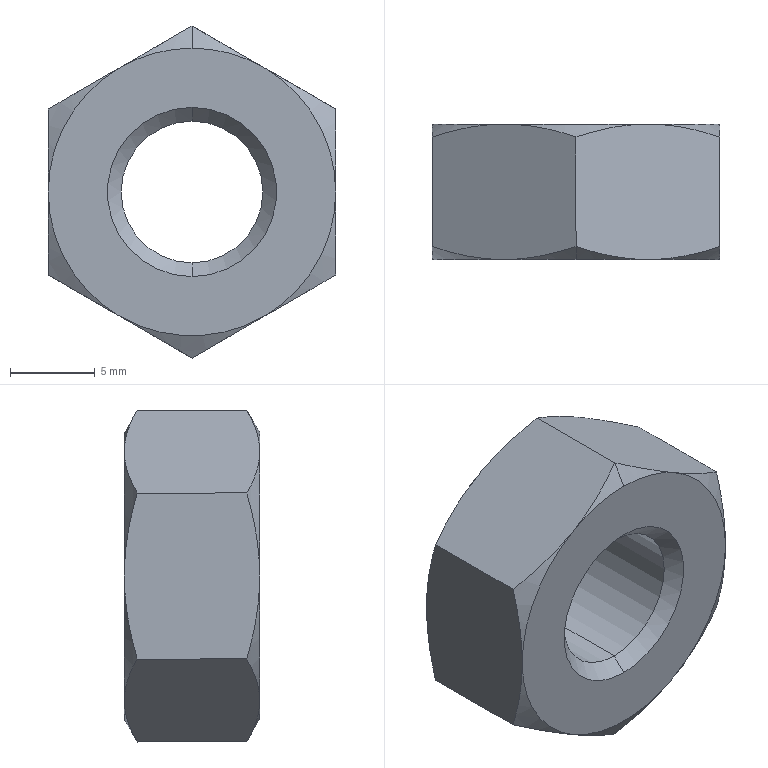Part | SolidWorks | features BaseBody 1 | 1 solid | 27 faces | box 17 x 8 x 19.63 mm | volume 1532 mm3 | cone 17 | plane 8 | cylinder 2 | commonest cylinder face diameters 8.376 x2
STEP:
#1=CARTESIAN_POINT('',(0.,0.812,-4.188));
#2=VERTEX_POINT('',#1);
#3=CARTESIAN_POINT('',(0.,0.812,4.188));
#4=VERTEX_POINT('',#3);
#5=CARTESIAN_POINT('',(0.,0.812,0.));
#6=DIRECTION('',(0.,1.,0.));
#7=DIRECTION('',(0.,0.,1.));
#8=AXIS2_PLACEMENT_3D('',#5,#6,#7);
#9=CIRCLE('',#8,4.188);
#10=EDGE_CURVE('',#2,#4,#9,.T.);
#11=ORIENTED_EDGE('',*,*,#10,.F.);
#12=CARTESIAN_POINT('',(0.,7.188,-4.188));
#13=VERTEX_POINT('',#12);
#14=CARTESIAN_POINT('',(0.,0.,-4.188));
#15=DIRECTION('',(0.,1.,0.));
#16=VECTOR('',#15,1000.);
#17=LINE('',#14,#16);
#18=EDGE_CURVE('',#2,#13,#17,.T.);
#19=ORIENTED_EDGE('',*,*,#18,.T.);
#20=CARTESIAN_POINT('',(0.,7.188,4.188));
#21=VERTEX_POINT('',#20);
#22=CARTESIAN_POINT('',(0.,7.188,0.));
#23=DIRECTION('',(0.,-1.,0.));
#24=DIRECTION('',(0.,0.,1.));
#25=AXIS2_PLACEMENT_3D('',#22,#23,#24);
#26=CIRCLE('',#25,4.188);
#27=EDGE_CURVE('',#21,#13,#26,.T.);
#28=ORIENTED_EDGE('',*,*,#27,.F.);
#29=CARTESIAN_POINT('',(0.,0.,4.188));
#30=DIRECTION('',(0.,1.,0.));
#31=VECTOR('',#30,1000.);
#32=LINE('',#29,#31);
#33=EDGE_CURVE('',#4,#21,#32,.T.);
#34=ORIENTED_EDGE('',*,*,#33,.F.);
#35=EDGE_LOOP('',(#11,#19,#28,#34));
#36=FACE_OUTER_BOUND('',#35,.T.);
#37=CARTESIAN_POINT('',(0.,0.,0.));
#38=DIRECTION('',(0.,1.,0.));
#39=DIRECTION('',(0.,0.,1.));
#40=AXIS2_PLACEMENT_3D('',#37,#38,#39);
#41=CYLINDRICAL_SURFACE('',#40,4.188);
#42=ADVANCED_FACE('',(#36),#41,.F.);
#43=ORIENTED_EDGE('',*,*,#27,.T.);
#44=CARTESIAN_POINT('',(0.,8.,-5.));
#45=VERTEX_POINT('',#44);
#46=CARTESIAN_POINT('',(0.,8.,-5.));
#47=DIRECTION('',(0.,0.7071,-0.7071));
#48=VECTOR('',#47,1000.);
#49=LINE('',#46,#48);
#50=EDGE_CURVE('',#13,#45,#49,.T.);
#51=ORIENTED_EDGE('',*,*,#50,.T.);
#52=CARTESIAN_POINT('',(0.,8.,5.));
#53=VERTEX_POINT('',#52);
#54=CARTESIAN_POINT('',(0.,8.,0.));
#55=DIRECTION('',(0.,-1.,0.));
#56=DIRECTION('',(0.,0.,1.));
#57=AXIS2_PLACEMENT_3D('',#54,#55,#56);
#58=CIRCLE('',#57,5.);
#59=EDGE_CURVE('',#53,#45,#58,.T.);
#60=ORIENTED_EDGE('',*,*,#59,.F.);
#61=CARTESIAN_POINT('',(0.,8.,5.));
#62=DIRECTION('',(0.,0.7071,0.7071));
#63=VECTOR('',#62,1000.);
#64=LINE('',#61,#63);
#65=EDGE_CURVE('',#21,#53,#64,.T.);
#66=ORIENTED_EDGE('',*,*,#65,.F.);
#67=EDGE_LOOP('',(#43,#51,#60,#66));
#68=FACE_OUTER_BOUND('',#67,.T.);
#69=CARTESIAN_POINT('',(0.,8.,0.));
#70=DIRECTION('',(0.,1.,0.));
#71=DIRECTION('',(0.,0.,1.));
#72=AXIS2_PLACEMENT_3D('',#69,#70,#71);
#73=CONICAL_SURFACE('',#72,5.,0.7854);
#74=ADVANCED_FACE('',(#68),#73,.F.);
#75=ORIENTED_EDGE('',*,*,#10,.T.);
#76=CARTESIAN_POINT('',(0.,0.,5.));
#77=VERTEX_POINT('',#76);
#78=CARTESIAN_POINT('',(0.,0.,5.));
#79=DIRECTION('',(0.,-0.7071,0.7071));
#80=VECTOR('',#79,1000.);
#81=LINE('',#78,#80);
#82=EDGE_CURVE('',#4,#77,#81,.T.);
#83=ORIENTED_EDGE('',*,*,#82,.T.);
#84=CARTESIAN_POINT('',(0.,0.,-5.));
#85=VERTEX_POINT('',#84);
#86=CARTESIAN_POINT('',(0.,0.,0.));
#87=DIRECTION('',(0.,1.,0.));
#88=DIRECTION('',(0.,0.,-1.));
#89=AXIS2_PLACEMENT_3D('',#86,#87,#88);
#90=CIRCLE('',#89,5.);
#91=EDGE_CURVE('',#85,#77,#90,.T.);
#92=ORIENTED_EDGE('',*,*,#91,.F.);
#93=CARTESIAN_POINT('',(0.,0.,-5.));
#94=DIRECTION('',(0.,-0.7071,-0.7071));
#95=VECTOR('',#94,1000.);
#96=LINE('',#93,#95);
#97=EDGE_CURVE('',#2,#85,#96,.T.);
#98=ORIENTED_EDGE('',*,*,#97,.F.);
#99=EDGE_LOOP('',(#75,#83,#92,#98));
#100=FACE_OUTER_BOUND('',#99,.T.);
#101=CARTESIAN_POINT('',(0.,0.,0.));
#102=DIRECTION('',(0.,-1.,0.));
#103=DIRECTION('',(0.,0.,-1.));
#104=AXIS2_PLACEMENT_3D('',#101,#102,#103);
#105=CONICAL_SURFACE('',#104,5.,0.7854);
#106=ADVANCED_FACE('',(#100),#105,.F.);
#107=CARTESIAN_POINT('',(-4.25,0.,7.361));
#108=VERTEX_POINT('',#107);
#109=CARTESIAN_POINT('',(0.,0.,8.5));
#110=VERTEX_POINT('',#109);
#111=CARTESIAN_POINT('',(0.,0.,0.));
#112=DIRECTION('',(0.,1.,0.));
#113=DIRECTION('',(0.,0.,1.));
#114=AXIS2_PLACEMENT_3D('',#111,#112,#113);
#115=CIRCLE('',#114,8.5);
#116=EDGE_CURVE('',#108,#110,#115,.T.);
#117=ORIENTED_EDGE('',*,*,#116,.T.);
#118=CARTESIAN_POINT('',(0.000000007,0.7592,9.815));
#119=VERTEX_POINT('',#118);
#120=CARTESIAN_POINT('',(0.,0.7637,9.823));
#121=DIRECTION('',(0.,0.5,0.866));
#122=VECTOR('',#121,1000.);
#123=LINE('',#120,#122);
#124=EDGE_CURVE('',#110,#119,#123,.T.);
#125=ORIENTED_EDGE('',*,*,#124,.T.);
#126=CARTESIAN_POINT('',(0.000000007,0.7592,9.815));
#127=CARTESIAN_POINT('',(-0.6943,0.5278,9.414));
#128=CARTESIAN_POINT('',(-1.394,0.3369,9.01));
#129=CARTESIAN_POINT('',(-2.809,0.07258,8.193));
#130=CARTESIAN_POINT('',(-3.525,0.,7.78));
#131=CARTESIAN_POINT('',(-4.25,0.,7.361));
#132=B_SPLINE_CURVE_WITH_KNOTS('',3,(#126,#127,#128,#129,#130,#131),.UNSPECIFIED.,.F.,.F.,(4,2,4),(0.,0.002483,0.004966),.UNSPECIFIED.);
#133=EDGE_CURVE('',#119,#108,#132,.T.);
#134=ORIENTED_EDGE('',*,*,#133,.T.);
#135=EDGE_LOOP('',(#117,#125,#134));
#136=FACE_OUTER_BOUND('',#135,.T.);
#137=CARTESIAN_POINT('',(0.,0.7637,0.));
#138=DIRECTION('',(0.,1.,0.));
#139=DIRECTION('',(0.,0.,1.));
#140=AXIS2_PLACEMENT_3D('',#137,#138,#139);
#141=CONICAL_SURFACE('',#140,9.823,1.047);
#142=ADVANCED_FACE('',(#136),#141,.T.);
#143=ORIENTED_EDGE('',*,*,#18,.F.);
#144=CARTESIAN_POINT('',(0.,0.812,0.));
#145=DIRECTION('',(0.,1.,0.));
#146=DIRECTION('',(0.,0.,1.));
#147=AXIS2_PLACEMENT_3D('',#144,#145,#146);
#148=CIRCLE('',#147,4.188);
#149=EDGE_CURVE('',#4,#2,#148,.T.);
#150=ORIENTED_EDGE('',*,*,#149,.F.);
#151=ORIENTED_EDGE('',*,*,#33,.T.);
#152=CARTESIAN_POINT('',(0.,7.188,0.));
#153=DIRECTION('',(0.,-1.,0.));
#154=DIRECTION('',(0.,0.,1.));
#155=AXIS2_PLACEMENT_3D('',#152,#153,#154);
#156=CIRCLE('',#155,4.188);
#157=EDGE_CURVE('',#13,#21,#156,.T.);
#158=ORIENTED_EDGE('',*,*,#157,.F.);
#159=EDGE_LOOP('',(#143,#150,#151,#158));
#160=FACE_OUTER_BOUND('',#159,.T.);
#161=CARTESIAN_POINT('',(0.,0.,0.));
#162=DIRECTION('',(0.,1.,0.));
#163=DIRECTION('',(0.,0.,1.));
#164=AXIS2_PLACEMENT_3D('',#161,#162,#163);
#165=CYLINDRICAL_SURFACE('',#164,4.188);
#166=ADVANCED_FACE('',(#160),#165,.F.);
#167=ORIENTED_EDGE('',*,*,#50,.F.);
#168=ORIENTED_EDGE('',*,*,#157,.T.);
#169=ORIENTED_EDGE('',*,*,#65,.T.);
#170=CARTESIAN_POINT('',(0.,8.,0.));
#171=DIRECTION('',(0.,-1.,0.));
#172=DIRECTION('',(0.,0.,1.));
#173=AXIS2_PLACEMENT_3D('',#170,#171,#172);
#174=CIRCLE('',#173,5.);
#175=EDGE_CURVE('',#45,#53,#174,.T.);
#176=ORIENTED_EDGE('',*,*,#175,.F.);
#177=EDGE_LOOP('',(#167,#168,#169,#176));
#178=FACE_OUTER_BOUND('',#177,.T.);
#179=CARTESIAN_POINT('',(0.,8.,0.));
#180=DIRECTION('',(0.,1.,0.));
#181=DIRECTION('',(0.,0.,1.));
#182=AXIS2_PLACEMENT_3D('',#179,#180,#181);
#183=CONICAL_SURFACE('',#182,5.,0.7854);
#184=ADVANCED_FACE('',(#178),#183,.F.);
#185=ORIENTED_EDGE('',*,*,#82,.F.);
#186=ORIENTED_EDGE('',*,*,#149,.T.);
#187=ORIENTED_EDGE('',*,*,#97,.T.);
#188=CARTESIAN_POINT('',(0.,0.,0.));
#189=DIRECTION('',(0.,1.,0.));
#190=DIRECTION('',(0.,0.,-1.));
#191=AXIS2_PLACEMENT_3D('',#188,#189,#190);
#192=CIRCLE('',#191,5.);
#193=EDGE_CURVE('',#77,#85,#192,.T.);
#194=ORIENTED_EDGE('',*,*,#193,.F.);
#195=EDGE_LOOP('',(#185,#186,#187,#194));
#196=FACE_OUTER_BOUND('',#195,.T.);
#197=CARTESIAN_POINT('',(0.,0.,0.));
#198=DIRECTION('',(0.,-1.,0.));
#199=DIRECTION('',(0.,0.,-1.));
#200=AXIS2_PLACEMENT_3D('',#197,#198,#199);
#201=CONICAL_SURFACE('',#200,5.,0.7854);
#202=ADVANCED_FACE('',(#196),#201,.F.);
#203=ORIENTED_EDGE('',*,*,#59,.T.);
#204=ORIENTED_EDGE('',*,*,#175,.T.);
#205=EDGE_LOOP('',(#203,#204));
#206=FACE_BOUND('',#205,.T.);
#207=CARTESIAN_POINT('',(4.25,8.,-7.361));
#208=VERTEX_POINT('',#207);
#209=CARTESIAN_POINT('',(8.5,8.,0.));
#210=VERTEX_POINT('',#209);
#211=CARTESIAN_POINT('',(0.,8.,0.));
#212=DIRECTION('',(0.,-1.,0.));
#213=DIRECTION('',(0.,0.,-1.));
#214=AXIS2_PLACEMENT_3D('',#211,#212,#213);
#215=CIRCLE('',#214,8.5);
#216=EDGE_CURVE('',#208,#210,#215,.T.);
#217=ORIENTED_EDGE('',*,*,#216,.F.);
#218=CARTESIAN_POINT('',(-4.25,8.,-7.361));
#219=VERTEX_POINT('',#218);
#220=CARTESIAN_POINT('',(0.,8.,0.));
#221=DIRECTION('',(0.,-1.,0.));
#222=DIRECTION('',(1.,0.,0.));
#223=AXIS2_PLACEMENT_3D('',#220,#221,#222);
#224=CIRCLE('',#223,8.5);
#225=EDGE_CURVE('',#219,#208,#224,.T.);
#226=ORIENTED_EDGE('',*,*,#225,.F.);
#227=CARTESIAN_POINT('',(-8.5,8.,0.));
#228=VERTEX_POINT('',#227);
#229=CARTESIAN_POINT('',(0.,8.,0.));
#230=DIRECTION('',(0.,-1.,0.));
#231=DIRECTION('',(0.,0.,-1.));
#232=AXIS2_PLACEMENT_3D('',#229,#230,#231);
#233=CIRCLE('',#232,8.5);
#234=EDGE_CURVE('',#228,#219,#233,.T.);
#235=ORIENTED_EDGE('',*,*,#234,.F.);
#236=CARTESIAN_POINT('',(-4.25,8.,7.361));
#237=VERTEX_POINT('',#236);
#238=CARTESIAN_POINT('',(0.,8.,0.));
#239=DIRECTION('',(0.,-1.,0.));
#240=DIRECTION('',(0.,0.,-1.));
#241=AXIS2_PLACEMENT_3D('',#238,#239,#240);
#242=CIRCLE('',#241,8.5);
#243=EDGE_CURVE('',#237,#228,#242,.T.);
#244=ORIENTED_EDGE('',*,*,#243,.F.);
#245=CARTESIAN_POINT('',(4.25,8.,7.361));
#246=VERTEX_POINT('',#245);
#247=CARTESIAN_POINT('',(0.,8.,0.));
#248=DIRECTION('',(0.,-1.,0.));
#249=DIRECTION('',(1.,0.,0.));
#250=AXIS2_PLACEMENT_3D('',#247,#248,#249);
#251=CIRCLE('',#250,8.5);
#252=EDGE_CURVE('',#246,#237,#251,.T.);
#253=ORIENTED_EDGE('',*,*,#252,.F.);
#254=CARTESIAN_POINT('',(0.,8.,0.));
#255=DIRECTION('',(0.,-1.,0.));
#256=DIRECTION('',(0.,0.,-1.));
#257=AXIS2_PLACEMENT_3D('',#254,#255,#256);
#258=CIRCLE('',#257,8.5);
#259=EDGE_CURVE('',#210,#246,#258,.T.);
#260=ORIENTED_EDGE('',*,*,#259,.F.);
#261=EDGE_LOOP('',(#217,#226,#235,#244,#253,#260));
#262=FACE_OUTER_BOUND('',#261,.T.);
#263=CARTESIAN_POINT('',(0.,8.,0.));
#264=DIRECTION('',(0.,-1.,0.));
#265=DIRECTION('',(0.,0.,-1.));
#266=AXIS2_PLACEMENT_3D('',#263,#264,#265);
#267=PLANE('',#266);
#268=ADVANCED_FACE('',(#206,#262),#267,.F.);
#269=CARTESIAN_POINT('',(4.25,0.,7.361));
#270=VERTEX_POINT('',#269);
#271=CARTESIAN_POINT('',(8.5,0.,0.));
#272=VERTEX_POINT('',#271);
#273=CARTESIAN_POINT('',(0.,0.,0.));
#274=DIRECTION('',(0.,1.,0.));
#275=DIRECTION('',(0.,0.,1.));
#276=AXIS2_PLACEMENT_3D('',#273,#274,#275);
#277=CIRCLE('',#276,8.5);
#278=EDGE_CURVE('',#270,#272,#277,.T.);
#279=ORIENTED_EDGE('',*,*,#278,.F.);
#280=CARTESIAN_POINT('',(0.,0.,0.));
#281=DIRECTION('',(0.,1.,0.));
#282=DIRECTION('',(0.,0.,1.));
#283=AXIS2_PLACEMENT_3D('',#280,#281,#282);
#284=CIRCLE('',#283,8.5);
#285=EDGE_CURVE('',#110,#270,#284,.T.);
#286=ORIENTED_EDGE('',*,*,#285,.F.);
#287=ORIENTED_EDGE('',*,*,#116,.F.);
#288=CARTESIAN_POINT('',(-8.5,0.,0.));
#289=VERTEX_POINT('',#288);
#290=CARTESIAN_POINT('',(0.,0.,0.));
#291=DIRECTION('',(0.,1.,0.));
#292=DIRECTION('',(0.,0.,1.));
#293=AXIS2_PLACEMENT_3D('',#290,#291,#292);
#294=CIRCLE('',#293,8.5);
#295=EDGE_CURVE('',#289,#108,#294,.T.);
#296=ORIENTED_EDGE('',*,*,#295,.F.);
#297=CARTESIAN_POINT('',(-4.25,0.,-7.361));
#298=VERTEX_POINT('',#297);
#299=CARTESIAN_POINT('',(0.,0.,0.));
#300=DIRECTION('',(0.,1.,0.));
#301=DIRECTION('',(0.,0.,1.));
#302=AXIS2_PLACEMENT_3D('',#299,#300,#301);
#303=CIRCLE('',#302,8.5);
#304=EDGE_CURVE('',#298,#289,#303,.T.);
#305=ORIENTED_EDGE('',*,*,#304,.F.);
#306=CARTESIAN_POINT('',(4.25,0.,-7.361));
#307=VERTEX_POINT('',#306);
#308=CARTESIAN_POINT('',(0.,0.,0.));
#309=DIRECTION('',(0.,1.,0.));
#310=DIRECTION('',(0.,0.,1.));
#311=AXIS2_PLACEMENT_3D('',#308,#309,#310);
#312=CIRCLE('',#311,8.5);
#313=EDGE_CURVE('',#307,#298,#312,.T.);
#314=ORIENTED_EDGE('',*,*,#313,.F.);
#315=CARTESIAN_POINT('',(0.,0.,0.));
#316=DIRECTION('',(0.,1.,0.));
#317=DIRECTION('',(0.,0.,1.));
#318=AXIS2_PLACEMENT_3D('',#315,#316,#317);
#319=CIRCLE('',#318,8.5);
#320=EDGE_CURVE('',#272,#307,#319,.T.);
#321=ORIENTED_EDGE('',*,*,#320,.F.);
#322=EDGE_LOOP('',(#279,#286,#287,#296,#305,#314,#321));
#323=FACE_OUTER_BOUND('',#322,.T.);
#324=ORIENTED_EDGE('',*,*,#91,.T.);
#325=ORIENTED_EDGE('',*,*,#193,.T.);
#326=EDGE_LOOP('',(#324,#325));
#327=FACE_BOUND('',#326,.T.);
#328=CARTESIAN_POINT('',(8.5,0.,0.));
#329=DIRECTION('',(0.,1.,0.));
#330=DIRECTION('',(0.,0.,1.));
#331=AXIS2_PLACEMENT_3D('',#328,#329,#330);
#332=PLANE('',#331);
#333=ADVANCED_FACE('',(#323,#327),#332,.F.);
#334=CARTESIAN_POINT('',(8.5,7.241,4.907));
#335=VERTEX_POINT('',#334);
#336=CARTESIAN_POINT('',(8.5,7.241,4.907));
#337=CARTESIAN_POINT('',(8.5,7.472,4.106));
#338=CARTESIAN_POINT('',(8.5,7.663,3.298));
#339=CARTESIAN_POINT('',(8.5,7.927,1.664));
#340=CARTESIAN_POINT('',(8.5,8.,0.8375));
#341=CARTESIAN_POINT('',(8.5,8.,0.));
#342=B_SPLINE_CURVE_WITH_KNOTS('',3,(#336,#337,#338,#339,#340,#341),.UNSPECIFIED.,.F.,.F.,(4,2,4),(0.,0.002483,0.004966),.UNSPECIFIED.);
#343=EDGE_CURVE('',#335,#210,#342,.T.);
#344=ORIENTED_EDGE('',*,*,#343,.T.);
#345=ORIENTED_EDGE('',*,*,#259,.T.);
#346=CARTESIAN_POINT('',(4.25,8.,7.361));
#347=CARTESIAN_POINT('',(4.975,8.,6.942));
#348=CARTESIAN_POINT('',(5.691,7.927,6.529));
#349=CARTESIAN_POINT('',(7.106,7.663,5.712));
#350=CARTESIAN_POINT('',(7.806,7.472,5.308));
#351=CARTESIAN_POINT('',(8.5,7.241,4.907));
#352=B_SPLINE_CURVE_WITH_KNOTS('',3,(#346,#347,#348,#349,#350,#351),.UNSPECIFIED.,.F.,.F.,(4,2,4),(0.,0.002483,0.004966),.UNSPECIFIED.);
#353=EDGE_CURVE('',#246,#335,#352,.T.);
#354=ORIENTED_EDGE('',*,*,#353,.T.);
#355=EDGE_LOOP('',(#344,#345,#354));
#356=FACE_OUTER_BOUND('',#355,.T.);
#357=CARTESIAN_POINT('',(0.,7.236,0.));
#358=DIRECTION('',(0.,-1.,0.));
#359=DIRECTION('',(0.,0.,-1.));
#360=AXIS2_PLACEMENT_3D('',#357,#358,#359);
#361=CONICAL_SURFACE('',#360,9.823,1.047);
#362=ADVANCED_FACE('',(#356),#361,.T.);
#363=CARTESIAN_POINT('',(8.5,7.241,-4.907));
#364=VERTEX_POINT('',#363);
#365=CARTESIAN_POINT('',(8.5,7.241,-4.907));
#366=CARTESIAN_POINT('',(7.806,7.472,-5.308));
#367=CARTESIAN_POINT('',(7.106,7.663,-5.712));
#368=CARTESIAN_POINT('',(5.691,7.927,-6.529));
#369=CARTESIAN_POINT('',(4.975,8.,-6.942));
#370=CARTESIAN_POINT('',(4.25,8.,-7.361));
#371=B_SPLINE_CURVE_WITH_KNOTS('',3,(#365,#366,#367,#368,#369,#370),.UNSPECIFIED.,.F.,.F.,(4,2,4),(0.,0.002483,0.004966),.UNSPECIFIED.);
#372=EDGE_CURVE('',#364,#208,#371,.T.);
#373=ORIENTED_EDGE('',*,*,#372,.T.);
#374=ORIENTED_EDGE('',*,*,#216,.T.);
#375=CARTESIAN_POINT('',(8.5,8.,0.));
#376=CARTESIAN_POINT('',(8.5,8.,-0.8375));
#377=CARTESIAN_POINT('',(8.5,7.927,-1.664));
#378=CARTESIAN_POINT('',(8.5,7.663,-3.298));
#379=CARTESIAN_POINT('',(8.5,7.472,-4.106));
#380=CARTESIAN_POINT('',(8.5,7.241,-4.907));
#381=B_SPLINE_CURVE_WITH_KNOTS('',3,(#375,#376,#377,#378,#379,#380),.UNSPECIFIED.,.F.,.F.,(4,2,4),(0.,0.002483,0.004966),.UNSPECIFIED.);
#382=EDGE_CURVE('',#210,#364,#381,.T.);
#383=ORIENTED_EDGE('',*,*,#382,.T.);
#384=EDGE_LOOP('',(#373,#374,#383));
#385=FACE_OUTER_BOUND('',#384,.T.);
#386=CARTESIAN_POINT('',(0.,7.236,0.));
#387=DIRECTION('',(0.,-1.,0.));
#388=DIRECTION('',(0.,0.,-1.));
#389=AXIS2_PLACEMENT_3D('',#386,#387,#388);
#390=CONICAL_SURFACE('',#389,9.823,1.047);
#391=ADVANCED_FACE('',(#385),#390,.T.);
#392=CARTESIAN_POINT('',(0.000000043,7.241,-9.815));
#393=VERTEX_POINT('',#392);
#394=CARTESIAN_POINT('',(4.25,8.,-7.361));
#395=CARTESIAN_POINT('',(3.525,8.,-7.78));
#396=CARTESIAN_POINT('',(2.809,7.927,-8.193));
#397=CARTESIAN_POINT('',(1.394,7.663,-9.01));
#398=CARTESIAN_POINT('',(0.6943,7.472,-9.414));
#399=CARTESIAN_POINT('',(0.000000043,7.241,-9.815));
#400=B_SPLINE_CURVE_WITH_KNOTS('',3,(#394,#395,#396,#397,#398,#399),.UNSPECIFIED.,.F.,.F.,(4,2,4),(0.,0.002483,0.004966),.UNSPECIFIED.);
#401=EDGE_CURVE('',#208,#393,#400,.T.);
#402=ORIENTED_EDGE('',*,*,#401,.T.);
#403=CARTESIAN_POINT('',(0.000000043,7.241,-9.815));
#404=CARTESIAN_POINT('',(-0.6943,7.472,-9.414));
#405=CARTESIAN_POINT('',(-1.394,7.663,-9.01));
#406=CARTESIAN_POINT('',(-2.809,7.927,-8.193));
#407=CARTESIAN_POINT('',(-3.525,8.,-7.78));
#408=CARTESIAN_POINT('',(-4.25,8.,-7.361));
#409=B_SPLINE_CURVE_WITH_KNOTS('',3,(#403,#404,#405,#406,#407,#408),.UNSPECIFIED.,.F.,.F.,(4,2,4),(0.,0.002483,0.004966),.UNSPECIFIED.);
#410=EDGE_CURVE('',#393,#219,#409,.T.);
#411=ORIENTED_EDGE('',*,*,#410,.T.);
#412=ORIENTED_EDGE('',*,*,#225,.T.);
#413=EDGE_LOOP('',(#402,#411,#412));
#414=FACE_OUTER_BOUND('',#413,.T.);
#415=CARTESIAN_POINT('',(0.,7.236,0.));
#416=DIRECTION('',(0.,-1.,0.));
#417=DIRECTION('',(1.,0.,0.));
#418=AXIS2_PLACEMENT_3D('',#415,#416,#417);
#419=CONICAL_SURFACE('',#418,9.823,1.047);
#420=ADVANCED_FACE('',(#414),#419,.T.);
#421=CARTESIAN_POINT('',(-8.5,7.241,-4.907));
#422=VERTEX_POINT('',#421);
#423=CARTESIAN_POINT('',(-4.25,8.,-7.361));
#424=CARTESIAN_POINT('',(-4.975,8.,-6.942));
#425=CARTESIAN_POINT('',(-5.691,7.927,-6.529));
#426=CARTESIAN_POINT('',(-7.106,7.663,-5.712));
#427=CARTESIAN_POINT('',(-7.806,7.472,-5.308));
#428=CARTESIAN_POINT('',(-8.5,7.241,-4.907));
#429=B_SPLINE_CURVE_WITH_KNOTS('',3,(#423,#424,#425,#426,#427,#428),.UNSPECIFIED.,.F.,.F.,(4,2,4),(0.,0.002483,0.004966),.UNSPECIFIED.);
#430=EDGE_CURVE('',#219,#422,#429,.T.);
#431=ORIENTED_EDGE('',*,*,#430,.T.);
#432=CARTESIAN_POINT('',(-8.5,7.241,-4.907));
#433=CARTESIAN_POINT('',(-8.5,7.472,-4.106));
#434=CARTESIAN_POINT('',(-8.5,7.663,-3.298));
#435=CARTESIAN_POINT('',(-8.5,7.927,-1.664));
#436=CARTESIAN_POINT('',(-8.5,8.,-0.8375));
#437=CARTESIAN_POINT('',(-8.5,8.,0.));
#438=B_SPLINE_CURVE_WITH_KNOTS('',3,(#432,#433,#434,#435,#436,#437),.UNSPECIFIED.,.F.,.F.,(4,2,4),(0.,0.002483,0.004966),.UNSPECIFIED.);
#439=EDGE_CURVE('',#422,#228,#438,.T.);
#440=ORIENTED_EDGE('',*,*,#439,.T.);
#441=ORIENTED_EDGE('',*,*,#234,.T.);
#442=EDGE_LOOP('',(#431,#440,#441));
#443=FACE_OUTER_BOUND('',#442,.T.);
#444=CARTESIAN_POINT('',(0.,7.236,0.));
#445=DIRECTION('',(0.,-1.,0.));
#446=DIRECTION('',(0.,0.,-1.));
#447=AXIS2_PLACEMENT_3D('',#444,#445,#446);
#448=CONICAL_SURFACE('',#447,9.823,1.047);
#449=ADVANCED_FACE('',(#443),#448,.T.);
#450=CARTESIAN_POINT('',(-8.5,7.241,4.907));
#451=VERTEX_POINT('',#450);
#452=CARTESIAN_POINT('',(-8.5,8.,0.));
#453=CARTESIAN_POINT('',(-8.5,8.,0.8375));
#454=CARTESIAN_POINT('',(-8.5,7.927,1.664));
#455=CARTESIAN_POINT('',(-8.5,7.663,3.298));
#456=CARTESIAN_POINT('',(-8.5,7.472,4.106));
#457=CARTESIAN_POINT('',(-8.5,7.241,4.907));
#458=B_SPLINE_CURVE_WITH_KNOTS('',3,(#452,#453,#454,#455,#456,#457),.UNSPECIFIED.,.F.,.F.,(4,2,4),(0.,0.002483,0.004966),.UNSPECIFIED.);
#459=EDGE_CURVE('',#228,#451,#458,.T.);
#460=ORIENTED_EDGE('',*,*,#459,.T.);
#461=CARTESIAN_POINT('',(-8.5,7.241,4.907));
#462=CARTESIAN_POINT('',(-7.806,7.472,5.308));
#463=CARTESIAN_POINT('',(-7.106,7.663,5.712));
#464=CARTESIAN_POINT('',(-5.691,7.927,6.529));
#465=CARTESIAN_POINT('',(-4.975,8.,6.942));
#466=CARTESIAN_POINT('',(-4.25,8.,7.361));
#467=B_SPLINE_CURVE_WITH_KNOTS('',3,(#461,#462,#463,#464,#465,#466),.UNSPECIFIED.,.F.,.F.,(4,2,4),(0.,0.002483,0.004966),.UNSPECIFIED.);
#468=EDGE_CURVE('',#451,#237,#467,.T.);
#469=ORIENTED_EDGE('',*,*,#468,.T.);
#470=ORIENTED_EDGE('',*,*,#243,.T.);
#471=EDGE_LOOP('',(#460,#469,#470));
#472=FACE_OUTER_BOUND('',#471,.T.);
#473=CARTESIAN_POINT('',(0.,7.236,0.));
#474=DIRECTION('',(0.,-1.,0.));
#475=DIRECTION('',(0.,0.,-1.));
#476=AXIS2_PLACEMENT_3D('',#473,#474,#475);
#477=CONICAL_SURFACE('',#476,9.823,1.047);
#478=ADVANCED_FACE('',(#472),#477,.T.);
#479=CARTESIAN_POINT('',(-0.000000043,7.241,9.815));
#480=VERTEX_POINT('',#479);
#481=CARTESIAN_POINT('',(-0.000000043,7.241,9.815));
#482=CARTESIAN_POINT('',(0.6943,7.472,9.414));
#483=CARTESIAN_POINT('',(1.394,7.663,9.01));
#484=CARTESIAN_POINT('',(2.809,7.927,8.193));
#485=CARTESIAN_POINT('',(3.525,8.,7.78));
#486=CARTESIAN_POINT('',(4.25,8.,7.361));
#487=B_SPLINE_CURVE_WITH_KNOTS('',3,(#481,#482,#483,#484,#485,#486),.UNSPECIFIED.,.F.,.F.,(4,2,4),(0.,0.002483,0.004966),.UNSPECIFIED.);
#488=EDGE_CURVE('',#480,#246,#487,.T.);
#489=ORIENTED_EDGE('',*,*,#488,.T.);
#490=ORIENTED_EDGE('',*,*,#252,.T.);
#491=CARTESIAN_POINT('',(-4.25,8.,7.361));
#492=CARTESIAN_POINT('',(-3.525,8.,7.78));
#493=CARTESIAN_POINT('',(-2.809,7.927,8.193));
#494=CARTESIAN_POINT('',(-1.394,7.663,9.01));
#495=CARTESIAN_POINT('',(-0.6943,7.472,9.414));
#496=CARTESIAN_POINT('',(-0.000000043,7.241,9.815));
#497=B_SPLINE_CURVE_WITH_KNOTS('',3,(#491,#492,#493,#494,#495,#496),.UNSPECIFIED.,.F.,.F.,(4,2,4),(0.,0.002483,0.004966),.UNSPECIFIED.);
#498=EDGE_CURVE('',#237,#480,#497,.T.);
#499=ORIENTED_EDGE('',*,*,#498,.T.);
#500=EDGE_LOOP('',(#489,#490,#499));
#501=FACE_OUTER_BOUND('',#500,.T.);
#502=CARTESIAN_POINT('',(0.,7.236,0.));
#503=DIRECTION('',(0.,-1.,0.));
#504=DIRECTION('',(1.,0.,0.));
#505=AXIS2_PLACEMENT_3D('',#502,#503,#504);
#506=CONICAL_SURFACE('',#505,9.823,1.047);
#507=ADVANCED_FACE('',(#501),#506,.T.);
#508=CARTESIAN_POINT('',(8.5,0.7592,-4.907));
#509=VERTEX_POINT('',#508);
#510=CARTESIAN_POINT('',(4.25,0.,-7.361));
#511=CARTESIAN_POINT('',(4.975,0.,-6.942));
#512=CARTESIAN_POINT('',(5.691,0.07258,-6.529));
#513=CARTESIAN_POINT('',(7.106,0.3369,-5.712));
#514=CARTESIAN_POINT('',(7.806,0.5278,-5.308));
#515=CARTESIAN_POINT('',(8.5,0.7592,-4.907));
#516=B_SPLINE_CURVE_WITH_KNOTS('',3,(#510,#511,#512,#513,#514,#515),.UNSPECIFIED.,.F.,.F.,(4,2,4),(0.,0.002483,0.004966),.UNSPECIFIED.);
#517=EDGE_CURVE('',#307,#509,#516,.T.);
#518=ORIENTED_EDGE('',*,*,#517,.T.);
#519=CARTESIAN_POINT('',(8.5,0.7592,-4.907));
#520=CARTESIAN_POINT('',(8.5,0.5278,-4.106));
#521=CARTESIAN_POINT('',(8.5,0.3369,-3.298));
#522=CARTESIAN_POINT('',(8.5,0.07258,-1.664));
#523=CARTESIAN_POINT('',(8.5,0.,-0.8375));
#524=CARTESIAN_POINT('',(8.5,0.,0.));
#525=B_SPLINE_CURVE_WITH_KNOTS('',3,(#519,#520,#521,#522,#523,#524),.UNSPECIFIED.,.F.,.F.,(4,2,4),(0.,0.002483,0.004966),.UNSPECIFIED.);
#526=EDGE_CURVE('',#509,#272,#525,.T.);
#527=ORIENTED_EDGE('',*,*,#526,.T.);
#528=ORIENTED_EDGE('',*,*,#320,.T.);
#529=EDGE_LOOP('',(#518,#527,#528));
#530=FACE_OUTER_BOUND('',#529,.T.);
#531=CARTESIAN_POINT('',(0.,0.7637,0.));
#532=DIRECTION('',(0.,1.,0.));
#533=DIRECTION('',(0.,0.,1.));
#534=AXIS2_PLACEMENT_3D('',#531,#532,#533);
#535=CONICAL_SURFACE('',#534,9.823,1.047);
#536=ADVANCED_FACE('',(#530),#535,.T.);
#537=CARTESIAN_POINT('',(8.5,0.7592,4.907));
#538=VERTEX_POINT('',#537);
#539=CARTESIAN_POINT('',(8.5,0.,0.));
#540=CARTESIAN_POINT('',(8.5,0.,0.8375));
#541=CARTESIAN_POINT('',(8.5,0.07258,1.664));
#542=CARTESIAN_POINT('',(8.5,0.3369,3.298));
#543=CARTESIAN_POINT('',(8.5,0.5278,4.106));
#544=CARTESIAN_POINT('',(8.5,0.7592,4.907));
#545=B_SPLINE_CURVE_WITH_KNOTS('',3,(#539,#540,#541,#542,#543,#544),.UNSPECIFIED.,.F.,.F.,(4,2,4),(0.,0.002483,0.004966),.UNSPECIFIED.);
#546=EDGE_CURVE('',#272,#538,#545,.T.);
#547=ORIENTED_EDGE('',*,*,#546,.T.);
#548=CARTESIAN_POINT('',(8.5,0.7592,4.907));
#549=CARTESIAN_POINT('',(7.806,0.5278,5.308));
#550=CARTESIAN_POINT('',(7.106,0.3369,5.712));
#551=CARTESIAN_POINT('',(5.691,0.07258,6.529));
#552=CARTESIAN_POINT('',(4.975,0.,6.942));
#553=CARTESIAN_POINT('',(4.25,0.,7.361));
#554=B_SPLINE_CURVE_WITH_KNOTS('',3,(#548,#549,#550,#551,#552,#553),.UNSPECIFIED.,.F.,.F.,(4,2,4),(0.,0.002483,0.004966),.UNSPECIFIED.);
#555=EDGE_CURVE('',#538,#270,#554,.T.);
#556=ORIENTED_EDGE('',*,*,#555,.T.);
#557=ORIENTED_EDGE('',*,*,#278,.T.);
#558=EDGE_LOOP('',(#547,#556,#557));
#559=FACE_OUTER_BOUND('',#558,.T.);
#560=CARTESIAN_POINT('',(0.,0.7637,0.));
#561=DIRECTION('',(0.,1.,0.));
#562=DIRECTION('',(0.,0.,1.));
#563=AXIS2_PLACEMENT_3D('',#560,#561,#562);
#564=CONICAL_SURFACE('',#563,9.823,1.047);
#565=ADVANCED_FACE('',(#559),#564,.T.);
#566=ORIENTED_EDGE('',*,*,#124,.F.);
#567=ORIENTED_EDGE('',*,*,#285,.T.);
#568=CARTESIAN_POINT('',(4.25,0.,7.361));
#569=CARTESIAN_POINT('',(3.525,0.,7.78));
#570=CARTESIAN_POINT('',(2.809,0.07258,8.193));
#571=CARTESIAN_POINT('',(1.394,0.3369,9.01));
#572=CARTESIAN_POINT('',(0.6943,0.5278,9.414));
#573=CARTESIAN_POINT('',(0.000000007,0.7592,9.815));
#574=B_SPLINE_CURVE_WITH_KNOTS('',3,(#568,#569,#570,#571,#572,#573),.UNSPECIFIED.,.F.,.F.,(4,2,4),(0.,0.002483,0.004966),.UNSPECIFIED.);
#575=EDGE_CURVE('',#270,#119,#574,.T.);
#576=ORIENTED_EDGE('',*,*,#575,.T.);
#577=EDGE_LOOP('',(#566,#567,#576));
#578=FACE_OUTER_BOUND('',#577,.T.);
#579=CARTESIAN_POINT('',(0.,0.7637,0.));
#580=DIRECTION('',(0.,1.,0.));
#581=DIRECTION('',(0.,0.,1.));
#582=AXIS2_PLACEMENT_3D('',#579,#580,#581);
#583=CONICAL_SURFACE('',#582,9.823,1.047);
#584=ADVANCED_FACE('',(#578),#583,.T.);
#585=CARTESIAN_POINT('',(-8.5,0.7592,4.907));
#586=VERTEX_POINT('',#585);
#587=CARTESIAN_POINT('',(-8.5,0.7592,4.907));
#588=CARTESIAN_POINT('',(-8.5,0.5278,4.106));
#589=CARTESIAN_POINT('',(-8.5,0.3369,3.298));
#590=CARTESIAN_POINT('',(-8.5,0.07258,1.664));
#591=CARTESIAN_POINT('',(-8.5,0.,0.8375));
#592=CARTESIAN_POINT('',(-8.5,0.,0.));
#593=B_SPLINE_CURVE_WITH_KNOTS('',3,(#587,#588,#589,#590,#591,#592),.UNSPECIFIED.,.F.,.F.,(4,2,4),(0.,0.002483,0.004966),.UNSPECIFIED.);
#594=EDGE_CURVE('',#586,#289,#593,.T.);
#595=ORIENTED_EDGE('',*,*,#594,.T.);
#596=ORIENTED_EDGE('',*,*,#295,.T.);
#597=CARTESIAN_POINT('',(-4.25,0.,7.361));
#598=CARTESIAN_POINT('',(-4.975,0.,6.942));
#599=CARTESIAN_POINT('',(-5.691,0.07258,6.529));
#600=CARTESIAN_POINT('',(-7.106,0.3369,5.712));
#601=CARTESIAN_POINT('',(-7.806,0.5278,5.308));
#602=CARTESIAN_POINT('',(-8.5,0.7592,4.907));
#603=B_SPLINE_CURVE_WITH_KNOTS('',3,(#597,#598,#599,#600,#601,#602),.UNSPECIFIED.,.F.,.F.,(4,2,4),(0.,0.002483,0.004966),.UNSPECIFIED.);
#604=EDGE_CURVE('',#108,#586,#603,.T.);
#605=ORIENTED_EDGE('',*,*,#604,.T.);
#606=EDGE_LOOP('',(#595,#596,#605));
#607=FACE_OUTER_BOUND('',#606,.T.);
#608=CARTESIAN_POINT('',(0.,0.7637,0.));
#609=DIRECTION('',(0.,1.,0.));
#610=DIRECTION('',(0.,0.,1.));
#611=AXIS2_PLACEMENT_3D('',#608,#609,#610);
#612=CONICAL_SURFACE('',#611,9.823,1.047);
#613=ADVANCED_FACE('',(#607),#612,.T.);
#614=CARTESIAN_POINT('',(-8.5,0.7592,-4.907));
#615=VERTEX_POINT('',#614);
#616=CARTESIAN_POINT('',(-8.5,0.,0.));
#617=CARTESIAN_POINT('',(-8.5,0.,-0.8375));
#618=CARTESIAN_POINT('',(-8.5,0.07258,-1.664));
#619=CARTESIAN_POINT('',(-8.5,0.3369,-3.298));
#620=CARTESIAN_POINT('',(-8.5,0.5278,-4.106));
#621=CARTESIAN_POINT('',(-8.5,0.7592,-4.907));
#622=B_SPLINE_CURVE_WITH_KNOTS('',3,(#616,#617,#618,#619,#620,#621),.UNSPECIFIED.,.F.,.F.,(4,2,4),(0.,0.002483,0.004966),.UNSPECIFIED.);
#623=EDGE_CURVE('',#289,#615,#622,.T.);
#624=ORIENTED_EDGE('',*,*,#623,.T.);
#625=CARTESIAN_POINT('',(-8.5,0.7592,-4.907));
#626=CARTESIAN_POINT('',(-7.806,0.5278,-5.308));
#627=CARTESIAN_POINT('',(-7.106,0.3369,-5.712));
#628=CARTESIAN_POINT('',(-5.691,0.07258,-6.529));
#629=CARTESIAN_POINT('',(-4.975,0.,-6.942));
#630=CARTESIAN_POINT('',(-4.25,0.,-7.361));
#631=B_SPLINE_CURVE_WITH_KNOTS('',3,(#625,#626,#627,#628,#629,#630),.UNSPECIFIED.,.F.,.F.,(4,2,4),(0.,0.002483,0.004966),.UNSPECIFIED.);
#632=EDGE_CURVE('',#615,#298,#631,.T.);
#633=ORIENTED_EDGE('',*,*,#632,.T.);
#634=ORIENTED_EDGE('',*,*,#304,.T.);
#635=EDGE_LOOP('',(#624,#633,#634));
#636=FACE_OUTER_BOUND('',#635,.T.);
#637=CARTESIAN_POINT('',(0.,0.7637,0.));
#638=DIRECTION('',(0.,1.,0.));
#639=DIRECTION('',(0.,0.,1.));
#640=AXIS2_PLACEMENT_3D('',#637,#638,#639);
#641=CONICAL_SURFACE('',#640,9.823,1.047);
#642=ADVANCED_FACE('',(#636),#641,.T.);
#643=CARTESIAN_POINT('',(-0.000000043,0.7592,-9.815));
#644=VERTEX_POINT('',#643);
#645=CARTESIAN_POINT('',(-4.25,0.,-7.361));
#646=CARTESIAN_POINT('',(-3.525,0.,-7.78));
#647=CARTESIAN_POINT('',(-2.809,0.07258,-8.193));
#648=CARTESIAN_POINT('',(-1.394,0.3369,-9.01));
#649=CARTESIAN_POINT('',(-0.6943,0.5278,-9.414));
#650=CARTESIAN_POINT('',(-0.000000043,0.7592,-9.815));
#651=B_SPLINE_CURVE_WITH_KNOTS('',3,(#645,#646,#647,#648,#649,#650),.UNSPECIFIED.,.F.,.F.,(4,2,4),(0.,0.002483,0.004966),.UNSPECIFIED.);
#652=EDGE_CURVE('',#298,#644,#651,.T.);
#653=ORIENTED_EDGE('',*,*,#652,.T.);
#654=CARTESIAN_POINT('',(-0.000000043,0.7592,-9.815));
#655=CARTESIAN_POINT('',(0.6943,0.5278,-9.414));
#656=CARTESIAN_POINT('',(1.394,0.3369,-9.01));
#657=CARTESIAN_POINT('',(2.809,0.07258,-8.193));
#658=CARTESIAN_POINT('',(3.525,0.,-7.78));
#659=CARTESIAN_POINT('',(4.25,0.,-7.361));
#660=B_SPLINE_CURVE_WITH_KNOTS('',3,(#654,#655,#656,#657,#658,#659),.UNSPECIFIED.,.F.,.F.,(4,2,4),(0.,0.002483,0.004966),.UNSPECIFIED.);
#661=EDGE_CURVE('',#644,#307,#660,.T.);
#662=ORIENTED_EDGE('',*,*,#661,.T.);
#663=ORIENTED_EDGE('',*,*,#313,.T.);
#664=EDGE_LOOP('',(#653,#662,#663));
#665=FACE_OUTER_BOUND('',#664,.T.);
#666=CARTESIAN_POINT('',(0.,0.7637,0.));
#667=DIRECTION('',(0.,1.,0.));
#668=DIRECTION('',(0.,0.,1.));
#669=AXIS2_PLACEMENT_3D('',#666,#667,#668);
#670=CONICAL_SURFACE('',#669,9.823,1.047);
#671=ADVANCED_FACE('',(#665),#670,.T.);
#672=ORIENTED_EDGE('',*,*,#546,.F.);
#673=ORIENTED_EDGE('',*,*,#526,.F.);
#674=CARTESIAN_POINT('',(8.5,8.,-4.907));
#675=DIRECTION('',(0.,-1.,0.));
#676=VECTOR('',#675,1000.);
#677=LINE('',#674,#676);
#678=EDGE_CURVE('',#364,#509,#677,.T.);
#679=ORIENTED_EDGE('',*,*,#678,.F.);
#680=ORIENTED_EDGE('',*,*,#382,.F.);
#681=ORIENTED_EDGE('',*,*,#343,.F.);
#682=CARTESIAN_POINT('',(8.5,8.,4.907));
#683=DIRECTION('',(0.,1.,0.));
#684=VECTOR('',#683,1000.);
#685=LINE('',#682,#684);
#686=EDGE_CURVE('',#538,#335,#685,.T.);
#687=ORIENTED_EDGE('',*,*,#686,.F.);
#688=EDGE_LOOP('',(#672,#673,#679,#680,#681,#687));
#689=FACE_OUTER_BOUND('',#688,.T.);
#690=CARTESIAN_POINT('',(8.5,8.,4.907));
#691=DIRECTION('',(-1.,0.,0.));
#692=DIRECTION('',(0.,0.,1.));
#693=AXIS2_PLACEMENT_3D('',#690,#691,#692);
#694=PLANE('',#693);
#695=ADVANCED_FACE('',(#689),#694,.F.);
#696=ORIENTED_EDGE('',*,*,#575,.F.);
#697=ORIENTED_EDGE('',*,*,#555,.F.);
#698=ORIENTED_EDGE('',*,*,#686,.T.);
#699=ORIENTED_EDGE('',*,*,#353,.F.);
#700=ORIENTED_EDGE('',*,*,#488,.F.);
#701=CARTESIAN_POINT('',(0.,8.,9.815));
#702=DIRECTION('',(0.,1.,0.));
#703=VECTOR('',#702,1000.);
#704=LINE('',#701,#703);
#705=EDGE_CURVE('',#119,#480,#704,.T.);
#706=ORIENTED_EDGE('',*,*,#705,.F.);
#707=EDGE_LOOP('',(#696,#697,#698,#699,#700,#706));
#708=FACE_OUTER_BOUND('',#707,.T.);
#709=CARTESIAN_POINT('',(0.,8.,9.815));
#710=DIRECTION('',(-0.5,0.,-0.866));
#711=DIRECTION('',(-0.866,0.,0.5));
#712=AXIS2_PLACEMENT_3D('',#709,#710,#711);
#713=PLANE('',#712);
#714=ADVANCED_FACE('',(#708),#713,.F.);
#715=ORIENTED_EDGE('',*,*,#517,.F.);
#716=ORIENTED_EDGE('',*,*,#661,.F.);
#717=CARTESIAN_POINT('',(0.,8.,-9.815));
#718=DIRECTION('',(0.,-1.,0.));
#719=VECTOR('',#718,1000.);
#720=LINE('',#717,#719);
#721=EDGE_CURVE('',#393,#644,#720,.T.);
#722=ORIENTED_EDGE('',*,*,#721,.F.);
#723=ORIENTED_EDGE('',*,*,#401,.F.);
#724=ORIENTED_EDGE('',*,*,#372,.F.);
#725=ORIENTED_EDGE('',*,*,#678,.T.);
#726=EDGE_LOOP('',(#715,#716,#722,#723,#724,#725));
#727=FACE_OUTER_BOUND('',#726,.T.);
#728=CARTESIAN_POINT('',(8.5,8.,-4.907));
#729=DIRECTION('',(-0.5,0.,0.866));
#730=DIRECTION('',(0.866,0.,0.5));
#731=AXIS2_PLACEMENT_3D('',#728,#729,#730);
#732=PLANE('',#731);
#733=ADVANCED_FACE('',(#727),#732,.F.);
#734=ORIENTED_EDGE('',*,*,#652,.F.);
#735=ORIENTED_EDGE('',*,*,#632,.F.);
#736=CARTESIAN_POINT('',(-8.5,8.,-4.907));
#737=DIRECTION('',(0.,-1.,0.));
#738=VECTOR('',#737,1000.);
#739=LINE('',#736,#738);
#740=EDGE_CURVE('',#422,#615,#739,.T.);
#741=ORIENTED_EDGE('',*,*,#740,.F.);
#742=ORIENTED_EDGE('',*,*,#430,.F.);
#743=ORIENTED_EDGE('',*,*,#410,.F.);
#744=ORIENTED_EDGE('',*,*,#721,.T.);
#745=EDGE_LOOP('',(#734,#735,#741,#742,#743,#744));
#746=FACE_OUTER_BOUND('',#745,.T.);
#747=CARTESIAN_POINT('',(0.,8.,-9.815));
#748=DIRECTION('',(0.5,0.,0.866));
#749=DIRECTION('',(0.866,0.,-0.5));
#750=AXIS2_PLACEMENT_3D('',#747,#748,#749);
#751=PLANE('',#750);
#752=ADVANCED_FACE('',(#746),#751,.F.);
#753=ORIENTED_EDGE('',*,*,#623,.F.);
#754=ORIENTED_EDGE('',*,*,#594,.F.);
#755=CARTESIAN_POINT('',(-8.5,8.,4.907));
#756=DIRECTION('',(0.,-1.,0.));
#757=VECTOR('',#756,1000.);
#758=LINE('',#755,#757);
#759=EDGE_CURVE('',#451,#586,#758,.T.);
#760=ORIENTED_EDGE('',*,*,#759,.F.);
#761=ORIENTED_EDGE('',*,*,#459,.F.);
#762=ORIENTED_EDGE('',*,*,#439,.F.);
#763=ORIENTED_EDGE('',*,*,#740,.T.);
#764=EDGE_LOOP('',(#753,#754,#760,#761,#762,#763));
#765=FACE_OUTER_BOUND('',#764,.T.);
#766=CARTESIAN_POINT('',(-8.5,8.,-4.907));
#767=DIRECTION('',(1.,0.,0.));
#768=DIRECTION('',(0.,0.,-1.));
#769=AXIS2_PLACEMENT_3D('',#766,#767,#768);
#770=PLANE('',#769);
#771=ADVANCED_FACE('',(#765),#770,.F.);
#772=ORIENTED_EDGE('',*,*,#604,.F.);
#773=ORIENTED_EDGE('',*,*,#133,.F.);
#774=ORIENTED_EDGE('',*,*,#705,.T.);
#775=ORIENTED_EDGE('',*,*,#498,.F.);
#776=ORIENTED_EDGE('',*,*,#468,.F.);
#777=ORIENTED_EDGE('',*,*,#759,.T.);
#778=EDGE_LOOP('',(#772,#773,#774,#775,#776,#777));
#779=FACE_OUTER_BOUND('',#778,.T.);
#780=CARTESIAN_POINT('',(-8.5,8.,4.907));
#781=DIRECTION('',(0.5,0.,-0.866));
#782=DIRECTION('',(-0.866,0.,-0.5));
#783=AXIS2_PLACEMENT_3D('',#780,#781,#782);
#784=PLANE('',#783);
#785=ADVANCED_FACE('',(#779),#784,.F.);
#786=CLOSED_SHELL('',(#42,#74,#106,#142,#166,#184,#202,#268,#333,#362,#391,#420,#449,#478,#507,#536,#565,#584,#613,#642,#671,#695,#714,#733,#752,#771,#785));
#787=MANIFOLD_SOLID_BREP('',#786);
#788=CARTESIAN_POINT('',(0.,0.,0.));
#789=DIRECTION('',(0.,0.,1.));
#790=DIRECTION('',(1.,0.,0.));
#791=AXIS2_PLACEMENT_3D('',#788,#789,#790);
#792=(LENGTH_UNIT()NAMED_UNIT(*)SI_UNIT(.MILLI.,.METRE.));
#793=UNCERTAINTY_MEASURE_WITH_UNIT(LENGTH_MEASURE(0.00001),#792,'','');
#794=(NAMED_UNIT(*)PLANE_ANGLE_UNIT()SI_UNIT($,.RADIAN.));
#795=(NAMED_UNIT(*)SI_UNIT($,.STERADIAN.)SOLID_ANGLE_UNIT());
#796=(GEOMETRIC_REPRESENTATION_CONTEXT(3)GLOBAL_UNCERTAINTY_ASSIGNED_CONTEXT((#793))GLOBAL_UNIT_ASSIGNED_CONTEXT((#792,#794,#795))REPRESENTATION_CONTEXT('',''));
#797=ADVANCED_BREP_SHAPE_REPRESENTATION('',(#787,#791),#796);